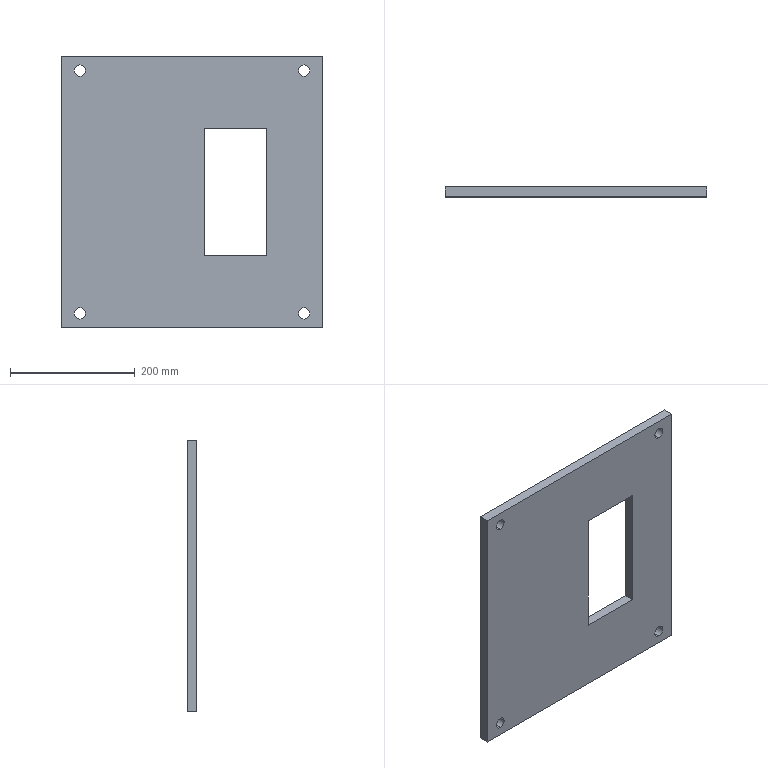Part | STEP file | 01-Base plate | 1 solid | 18 faces | box 420 x 16 x 435 mm | volume 2578914 mm3 | plane 10 | cylinder 8 | commonest cylinder face diameters 18 x8
STEP:
#1=CARTESIAN_POINT('',(0.,0.,0.));
#2=DIRECTION('',(0.,0.,1.));
#3=DIRECTION('',(1.,0.,0.));
#4=AXIS2_PLACEMENT_3D('',#1,#2,#3);
#5=CARTESIAN_POINT('',(30.,0.,421.5));
#6=VERTEX_POINT('',#5);
#7=CARTESIAN_POINT('',(30.,16.,421.5));
#8=VERTEX_POINT('',#7);
#9=CARTESIAN_POINT('',(30.,-14.,421.5));
#10=DIRECTION('',(0.,1.,0.));
#11=VECTOR('',#10,1.);
#12=LINE('',#9,#11);
#13=CARTESIAN_POINT('',(30.,-14.,412.5));
#14=DIRECTION('',(0.,1.,0.));
#15=DIRECTION('',(0.,0.,1.));
#16=AXIS2_PLACEMENT_3D('',#13,#14,#15);
#17=CYLINDRICAL_SURFACE('',#16,9.);
#18=CARTESIAN_POINT('',(6.283,0.));
#19=DIRECTION('',(0.,1.));
#20=VECTOR('',#19,1.);
#21=LINE('',#18,#20);
#22=(GEOMETRIC_REPRESENTATION_CONTEXT(2)PARAMETRIC_REPRESENTATION_CONTEXT()REPRESENTATION_CONTEXT('',''));
#23=DEFINITIONAL_REPRESENTATION('',(#21),#22);
#24=PCURVE('',#17,#23);
#25=CARTESIAN_POINT('',(30.,-14.,412.5));
#26=DIRECTION('',(0.,1.,0.));
#27=DIRECTION('',(0.,0.,1.));
#28=AXIS2_PLACEMENT_3D('',#25,#26,#27);
#29=CYLINDRICAL_SURFACE('',#28,9.);
#30=CARTESIAN_POINT('',(0.,0.));
#31=DIRECTION('',(0.,1.));
#32=VECTOR('',#31,1.);
#33=LINE('',#30,#32);
#34=(GEOMETRIC_REPRESENTATION_CONTEXT(2)PARAMETRIC_REPRESENTATION_CONTEXT()REPRESENTATION_CONTEXT('',''));
#35=DEFINITIONAL_REPRESENTATION('',(#33),#34);
#36=PCURVE('',#29,#35);
#37=SURFACE_CURVE('',#12,(#24,#36),.PCURVE_S1.);
#38=EDGE_CURVE('',#6,#8,#37,.T.);
#39=ORIENTED_EDGE('',*,*,#38,.T.);
#40=CARTESIAN_POINT('',(30.,16.,403.5));
#41=VERTEX_POINT('',#40);
#42=CARTESIAN_POINT('',(30.,16.,412.5));
#43=DIRECTION('',(0.,1.,0.));
#44=DIRECTION('',(0.,0.,1.));
#45=AXIS2_PLACEMENT_3D('',#42,#43,#44);
#46=CIRCLE('',#45,9.);
#47=CARTESIAN_POINT('',(0.,30.));
#48=DIRECTION('',(1.,0.));
#49=VECTOR('',#48,1.);
#50=LINE('',#47,#49);
#51=(GEOMETRIC_REPRESENTATION_CONTEXT(2)PARAMETRIC_REPRESENTATION_CONTEXT()REPRESENTATION_CONTEXT('',''));
#52=DEFINITIONAL_REPRESENTATION('',(#50),#51);
#53=PCURVE('',#17,#52);
#54=CARTESIAN_POINT('',(0.,16.,0.));
#55=DIRECTION('',(0.,1.,0.));
#56=DIRECTION('',(0.,0.,1.));
#57=AXIS2_PLACEMENT_3D('',#54,#55,#56);
#58=PLANE('',#57);
#59=CARTESIAN_POINT('',(412.5,30.));
#60=DIRECTION('',(1.,0.));
#61=AXIS2_PLACEMENT_2D('',#59,#60);
#62=CIRCLE('',#61,9.);
#63=(GEOMETRIC_REPRESENTATION_CONTEXT(2)PARAMETRIC_REPRESENTATION_CONTEXT()REPRESENTATION_CONTEXT('',''));
#64=DEFINITIONAL_REPRESENTATION('',(#62),#63);
#65=PCURVE('',#58,#64);
#66=SURFACE_CURVE('',#46,(#53,#65),.PCURVE_S1.);
#67=EDGE_CURVE('',#41,#8,#66,.T.);
#68=ORIENTED_EDGE('',*,*,#67,.F.);
#69=CARTESIAN_POINT('',(30.,0.,403.5));
#70=VERTEX_POINT('',#69);
#71=CARTESIAN_POINT('',(30.,-14.,403.5));
#72=DIRECTION('',(0.,1.,0.));
#73=VECTOR('',#72,1.);
#74=LINE('',#71,#73);
#75=CARTESIAN_POINT('',(3.142,0.));
#76=DIRECTION('',(0.,1.));
#77=VECTOR('',#76,1.);
#78=LINE('',#75,#77);
#79=(GEOMETRIC_REPRESENTATION_CONTEXT(2)PARAMETRIC_REPRESENTATION_CONTEXT()REPRESENTATION_CONTEXT('',''));
#80=DEFINITIONAL_REPRESENTATION('',(#78),#79);
#81=PCURVE('',#17,#80);
#82=CARTESIAN_POINT('',(3.142,0.));
#83=DIRECTION('',(0.,1.));
#84=VECTOR('',#83,1.);
#85=LINE('',#82,#84);
#86=(GEOMETRIC_REPRESENTATION_CONTEXT(2)PARAMETRIC_REPRESENTATION_CONTEXT()REPRESENTATION_CONTEXT('',''));
#87=DEFINITIONAL_REPRESENTATION('',(#85),#86);
#88=PCURVE('',#29,#87);
#89=SURFACE_CURVE('',#74,(#81,#88),.PCURVE_S1.);
#90=EDGE_CURVE('',#70,#41,#89,.T.);
#91=ORIENTED_EDGE('',*,*,#90,.F.);
#92=CARTESIAN_POINT('',(30.,0.,412.5));
#93=DIRECTION('',(0.,1.,0.));
#94=DIRECTION('',(0.,0.,1.));
#95=AXIS2_PLACEMENT_3D('',#92,#93,#94);
#96=CIRCLE('',#95,9.);
#97=CARTESIAN_POINT('',(0.,14.));
#98=DIRECTION('',(1.,0.));
#99=VECTOR('',#98,1.);
#100=LINE('',#97,#99);
#101=(GEOMETRIC_REPRESENTATION_CONTEXT(2)PARAMETRIC_REPRESENTATION_CONTEXT()REPRESENTATION_CONTEXT('',''));
#102=DEFINITIONAL_REPRESENTATION('',(#100),#101);
#103=PCURVE('',#17,#102);
#104=CARTESIAN_POINT('',(0.,0.,0.));
#105=DIRECTION('',(0.,1.,0.));
#106=DIRECTION('',(0.,0.,1.));
#107=AXIS2_PLACEMENT_3D('',#104,#105,#106);
#108=PLANE('',#107);
#109=CARTESIAN_POINT('',(412.5,30.));
#110=DIRECTION('',(1.,0.));
#111=AXIS2_PLACEMENT_2D('',#109,#110);
#112=CIRCLE('',#111,9.);
#113=(GEOMETRIC_REPRESENTATION_CONTEXT(2)PARAMETRIC_REPRESENTATION_CONTEXT()REPRESENTATION_CONTEXT('',''));
#114=DEFINITIONAL_REPRESENTATION('',(#112),#113);
#115=PCURVE('',#108,#114);
#116=SURFACE_CURVE('',#96,(#103,#115),.PCURVE_S1.);
#117=EDGE_CURVE('',#70,#6,#116,.T.);
#118=ORIENTED_EDGE('',*,*,#117,.T.);
#119=EDGE_LOOP('',(#39,#68,#91,#118));
#120=FACE_BOUND('',#119,.F.);
#121=ADVANCED_FACE('',(#120),#17,.F.);
#122=CARTESIAN_POINT('',(390.,0.,421.5));
#123=VERTEX_POINT('',#122);
#124=CARTESIAN_POINT('',(390.,16.,421.5));
#125=VERTEX_POINT('',#124);
#126=CARTESIAN_POINT('',(390.,-14.,421.5));
#127=DIRECTION('',(0.,1.,0.));
#128=VECTOR('',#127,1.);
#129=LINE('',#126,#128);
#130=CARTESIAN_POINT('',(390.,-14.,412.5));
#131=DIRECTION('',(0.,1.,0.));
#132=DIRECTION('',(0.,0.,1.));
#133=AXIS2_PLACEMENT_3D('',#130,#131,#132);
#134=CYLINDRICAL_SURFACE('',#133,9.);
#135=CARTESIAN_POINT('',(6.283,0.));
#136=DIRECTION('',(0.,1.));
#137=VECTOR('',#136,1.);
#138=LINE('',#135,#137);
#139=(GEOMETRIC_REPRESENTATION_CONTEXT(2)PARAMETRIC_REPRESENTATION_CONTEXT()REPRESENTATION_CONTEXT('',''));
#140=DEFINITIONAL_REPRESENTATION('',(#138),#139);
#141=PCURVE('',#134,#140);
#142=CARTESIAN_POINT('',(390.,-14.,412.5));
#143=DIRECTION('',(0.,1.,0.));
#144=DIRECTION('',(0.,0.,1.));
#145=AXIS2_PLACEMENT_3D('',#142,#143,#144);
#146=CYLINDRICAL_SURFACE('',#145,9.);
#147=CARTESIAN_POINT('',(0.,0.));
#148=DIRECTION('',(0.,1.));
#149=VECTOR('',#148,1.);
#150=LINE('',#147,#149);
#151=(GEOMETRIC_REPRESENTATION_CONTEXT(2)PARAMETRIC_REPRESENTATION_CONTEXT()REPRESENTATION_CONTEXT('',''));
#152=DEFINITIONAL_REPRESENTATION('',(#150),#151);
#153=PCURVE('',#146,#152);
#154=SURFACE_CURVE('',#129,(#141,#153),.PCURVE_S1.);
#155=EDGE_CURVE('',#123,#125,#154,.T.);
#156=ORIENTED_EDGE('',*,*,#155,.T.);
#157=CARTESIAN_POINT('',(390.,16.,403.5));
#158=VERTEX_POINT('',#157);
#159=CARTESIAN_POINT('',(390.,16.,412.5));
#160=DIRECTION('',(0.,1.,0.));
#161=DIRECTION('',(0.,0.,1.));
#162=AXIS2_PLACEMENT_3D('',#159,#160,#161);
#163=CIRCLE('',#162,9.);
#164=CARTESIAN_POINT('',(0.,30.));
#165=DIRECTION('',(1.,0.));
#166=VECTOR('',#165,1.);
#167=LINE('',#164,#166);
#168=(GEOMETRIC_REPRESENTATION_CONTEXT(2)PARAMETRIC_REPRESENTATION_CONTEXT()REPRESENTATION_CONTEXT('',''));
#169=DEFINITIONAL_REPRESENTATION('',(#167),#168);
#170=PCURVE('',#134,#169);
#171=CARTESIAN_POINT('',(412.5,390.));
#172=DIRECTION('',(1.,0.));
#173=AXIS2_PLACEMENT_2D('',#171,#172);
#174=CIRCLE('',#173,9.);
#175=(GEOMETRIC_REPRESENTATION_CONTEXT(2)PARAMETRIC_REPRESENTATION_CONTEXT()REPRESENTATION_CONTEXT('',''));
#176=DEFINITIONAL_REPRESENTATION('',(#174),#175);
#177=PCURVE('',#58,#176);
#178=SURFACE_CURVE('',#163,(#170,#177),.PCURVE_S1.);
#179=EDGE_CURVE('',#158,#125,#178,.T.);
#180=ORIENTED_EDGE('',*,*,#179,.F.);
#181=CARTESIAN_POINT('',(390.,0.,403.5));
#182=VERTEX_POINT('',#181);
#183=CARTESIAN_POINT('',(390.,-14.,403.5));
#184=DIRECTION('',(0.,1.,0.));
#185=VECTOR('',#184,1.);
#186=LINE('',#183,#185);
#187=CARTESIAN_POINT('',(3.142,0.));
#188=DIRECTION('',(0.,1.));
#189=VECTOR('',#188,1.);
#190=LINE('',#187,#189);
#191=(GEOMETRIC_REPRESENTATION_CONTEXT(2)PARAMETRIC_REPRESENTATION_CONTEXT()REPRESENTATION_CONTEXT('',''));
#192=DEFINITIONAL_REPRESENTATION('',(#190),#191);
#193=PCURVE('',#134,#192);
#194=CARTESIAN_POINT('',(3.142,0.));
#195=DIRECTION('',(0.,1.));
#196=VECTOR('',#195,1.);
#197=LINE('',#194,#196);
#198=(GEOMETRIC_REPRESENTATION_CONTEXT(2)PARAMETRIC_REPRESENTATION_CONTEXT()REPRESENTATION_CONTEXT('',''));
#199=DEFINITIONAL_REPRESENTATION('',(#197),#198);
#200=PCURVE('',#146,#199);
#201=SURFACE_CURVE('',#186,(#193,#200),.PCURVE_S1.);
#202=EDGE_CURVE('',#182,#158,#201,.T.);
#203=ORIENTED_EDGE('',*,*,#202,.F.);
#204=CARTESIAN_POINT('',(390.,0.,412.5));
#205=DIRECTION('',(0.,1.,0.));
#206=DIRECTION('',(0.,0.,1.));
#207=AXIS2_PLACEMENT_3D('',#204,#205,#206);
#208=CIRCLE('',#207,9.);
#209=CARTESIAN_POINT('',(0.,14.));
#210=DIRECTION('',(1.,0.));
#211=VECTOR('',#210,1.);
#212=LINE('',#209,#211);
#213=(GEOMETRIC_REPRESENTATION_CONTEXT(2)PARAMETRIC_REPRESENTATION_CONTEXT()REPRESENTATION_CONTEXT('',''));
#214=DEFINITIONAL_REPRESENTATION('',(#212),#213);
#215=PCURVE('',#134,#214);
#216=CARTESIAN_POINT('',(412.5,390.));
#217=DIRECTION('',(1.,0.));
#218=AXIS2_PLACEMENT_2D('',#216,#217);
#219=CIRCLE('',#218,9.);
#220=(GEOMETRIC_REPRESENTATION_CONTEXT(2)PARAMETRIC_REPRESENTATION_CONTEXT()REPRESENTATION_CONTEXT('',''));
#221=DEFINITIONAL_REPRESENTATION('',(#219),#220);
#222=PCURVE('',#108,#221);
#223=SURFACE_CURVE('',#208,(#215,#222),.PCURVE_S1.);
#224=EDGE_CURVE('',#182,#123,#223,.T.);
#225=ORIENTED_EDGE('',*,*,#224,.T.);
#226=EDGE_LOOP('',(#156,#180,#203,#225));
#227=FACE_BOUND('',#226,.F.);
#228=ADVANCED_FACE('',(#227),#134,.F.);
#229=CARTESIAN_POINT('',(390.,0.,31.5));
#230=VERTEX_POINT('',#229);
#231=CARTESIAN_POINT('',(390.,16.,31.5));
#232=VERTEX_POINT('',#231);
#233=CARTESIAN_POINT('',(390.,-14.,31.5));
#234=DIRECTION('',(0.,1.,0.));
#235=VECTOR('',#234,1.);
#236=LINE('',#233,#235);
#237=CARTESIAN_POINT('',(390.,-14.,22.5));
#238=DIRECTION('',(0.,1.,0.));
#239=DIRECTION('',(0.,0.,1.));
#240=AXIS2_PLACEMENT_3D('',#237,#238,#239);
#241=CYLINDRICAL_SURFACE('',#240,9.);
#242=CARTESIAN_POINT('',(6.283,0.));
#243=DIRECTION('',(0.,1.));
#244=VECTOR('',#243,1.);
#245=LINE('',#242,#244);
#246=(GEOMETRIC_REPRESENTATION_CONTEXT(2)PARAMETRIC_REPRESENTATION_CONTEXT()REPRESENTATION_CONTEXT('',''));
#247=DEFINITIONAL_REPRESENTATION('',(#245),#246);
#248=PCURVE('',#241,#247);
#249=CARTESIAN_POINT('',(390.,-14.,22.5));
#250=DIRECTION('',(0.,1.,0.));
#251=DIRECTION('',(0.,0.,1.));
#252=AXIS2_PLACEMENT_3D('',#249,#250,#251);
#253=CYLINDRICAL_SURFACE('',#252,9.);
#254=CARTESIAN_POINT('',(0.,0.));
#255=DIRECTION('',(0.,1.));
#256=VECTOR('',#255,1.);
#257=LINE('',#254,#256);
#258=(GEOMETRIC_REPRESENTATION_CONTEXT(2)PARAMETRIC_REPRESENTATION_CONTEXT()REPRESENTATION_CONTEXT('',''));
#259=DEFINITIONAL_REPRESENTATION('',(#257),#258);
#260=PCURVE('',#253,#259);
#261=SURFACE_CURVE('',#236,(#248,#260),.PCURVE_S1.);
#262=EDGE_CURVE('',#230,#232,#261,.T.);
#263=ORIENTED_EDGE('',*,*,#262,.T.);
#264=CARTESIAN_POINT('',(390.,16.,13.5));
#265=VERTEX_POINT('',#264);
#266=CARTESIAN_POINT('',(390.,16.,22.5));
#267=DIRECTION('',(0.,1.,0.));
#268=DIRECTION('',(0.,0.,1.));
#269=AXIS2_PLACEMENT_3D('',#266,#267,#268);
#270=CIRCLE('',#269,9.);
#271=CARTESIAN_POINT('',(0.,30.));
#272=DIRECTION('',(1.,0.));
#273=VECTOR('',#272,1.);
#274=LINE('',#271,#273);
#275=(GEOMETRIC_REPRESENTATION_CONTEXT(2)PARAMETRIC_REPRESENTATION_CONTEXT()REPRESENTATION_CONTEXT('',''));
#276=DEFINITIONAL_REPRESENTATION('',(#274),#275);
#277=PCURVE('',#241,#276);
#278=CARTESIAN_POINT('',(22.5,390.));
#279=DIRECTION('',(1.,0.));
#280=AXIS2_PLACEMENT_2D('',#278,#279);
#281=CIRCLE('',#280,9.);
#282=(GEOMETRIC_REPRESENTATION_CONTEXT(2)PARAMETRIC_REPRESENTATION_CONTEXT()REPRESENTATION_CONTEXT('',''));
#283=DEFINITIONAL_REPRESENTATION('',(#281),#282);
#284=PCURVE('',#58,#283);
#285=SURFACE_CURVE('',#270,(#277,#284),.PCURVE_S1.);
#286=EDGE_CURVE('',#265,#232,#285,.T.);
#287=ORIENTED_EDGE('',*,*,#286,.F.);
#288=CARTESIAN_POINT('',(390.,0.,13.5));
#289=VERTEX_POINT('',#288);
#290=CARTESIAN_POINT('',(390.,-14.,13.5));
#291=DIRECTION('',(0.,1.,0.));
#292=VECTOR('',#291,1.);
#293=LINE('',#290,#292);
#294=CARTESIAN_POINT('',(3.142,0.));
#295=DIRECTION('',(0.,1.));
#296=VECTOR('',#295,1.);
#297=LINE('',#294,#296);
#298=(GEOMETRIC_REPRESENTATION_CONTEXT(2)PARAMETRIC_REPRESENTATION_CONTEXT()REPRESENTATION_CONTEXT('',''));
#299=DEFINITIONAL_REPRESENTATION('',(#297),#298);
#300=PCURVE('',#241,#299);
#301=CARTESIAN_POINT('',(3.142,0.));
#302=DIRECTION('',(0.,1.));
#303=VECTOR('',#302,1.);
#304=LINE('',#301,#303);
#305=(GEOMETRIC_REPRESENTATION_CONTEXT(2)PARAMETRIC_REPRESENTATION_CONTEXT()REPRESENTATION_CONTEXT('',''));
#306=DEFINITIONAL_REPRESENTATION('',(#304),#305);
#307=PCURVE('',#253,#306);
#308=SURFACE_CURVE('',#293,(#300,#307),.PCURVE_S1.);
#309=EDGE_CURVE('',#289,#265,#308,.T.);
#310=ORIENTED_EDGE('',*,*,#309,.F.);
#311=CARTESIAN_POINT('',(390.,0.,22.5));
#312=DIRECTION('',(0.,1.,0.));
#313=DIRECTION('',(0.,0.,1.));
#314=AXIS2_PLACEMENT_3D('',#311,#312,#313);
#315=CIRCLE('',#314,9.);
#316=CARTESIAN_POINT('',(0.,14.));
#317=DIRECTION('',(1.,0.));
#318=VECTOR('',#317,1.);
#319=LINE('',#316,#318);
#320=(GEOMETRIC_REPRESENTATION_CONTEXT(2)PARAMETRIC_REPRESENTATION_CONTEXT()REPRESENTATION_CONTEXT('',''));
#321=DEFINITIONAL_REPRESENTATION('',(#319),#320);
#322=PCURVE('',#241,#321);
#323=CARTESIAN_POINT('',(22.5,390.));
#324=DIRECTION('',(1.,0.));
#325=AXIS2_PLACEMENT_2D('',#323,#324);
#326=CIRCLE('',#325,9.);
#327=(GEOMETRIC_REPRESENTATION_CONTEXT(2)PARAMETRIC_REPRESENTATION_CONTEXT()REPRESENTATION_CONTEXT('',''));
#328=DEFINITIONAL_REPRESENTATION('',(#326),#327);
#329=PCURVE('',#108,#328);
#330=SURFACE_CURVE('',#315,(#322,#329),.PCURVE_S1.);
#331=EDGE_CURVE('',#289,#230,#330,.T.);
#332=ORIENTED_EDGE('',*,*,#331,.T.);
#333=EDGE_LOOP('',(#263,#287,#310,#332));
#334=FACE_BOUND('',#333,.F.);
#335=ADVANCED_FACE('',(#334),#241,.F.);
#336=CARTESIAN_POINT('',(30.,0.,31.5));
#337=VERTEX_POINT('',#336);
#338=CARTESIAN_POINT('',(30.,16.,31.5));
#339=VERTEX_POINT('',#338);
#340=CARTESIAN_POINT('',(30.,-14.,31.5));
#341=DIRECTION('',(0.,1.,0.));
#342=VECTOR('',#341,1.);
#343=LINE('',#340,#342);
#344=CARTESIAN_POINT('',(30.,-14.,22.5));
#345=DIRECTION('',(0.,1.,0.));
#346=DIRECTION('',(0.,0.,1.));
#347=AXIS2_PLACEMENT_3D('',#344,#345,#346);
#348=CYLINDRICAL_SURFACE('',#347,9.);
#349=CARTESIAN_POINT('',(6.283,0.));
#350=DIRECTION('',(0.,1.));
#351=VECTOR('',#350,1.);
#352=LINE('',#349,#351);
#353=(GEOMETRIC_REPRESENTATION_CONTEXT(2)PARAMETRIC_REPRESENTATION_CONTEXT()REPRESENTATION_CONTEXT('',''));
#354=DEFINITIONAL_REPRESENTATION('',(#352),#353);
#355=PCURVE('',#348,#354);
#356=CARTESIAN_POINT('',(30.,-14.,22.5));
#357=DIRECTION('',(0.,1.,0.));
#358=DIRECTION('',(0.,0.,1.));
#359=AXIS2_PLACEMENT_3D('',#356,#357,#358);
#360=CYLINDRICAL_SURFACE('',#359,9.);
#361=CARTESIAN_POINT('',(0.,0.));
#362=DIRECTION('',(0.,1.));
#363=VECTOR('',#362,1.);
#364=LINE('',#361,#363);
#365=(GEOMETRIC_REPRESENTATION_CONTEXT(2)PARAMETRIC_REPRESENTATION_CONTEXT()REPRESENTATION_CONTEXT('',''));
#366=DEFINITIONAL_REPRESENTATION('',(#364),#365);
#367=PCURVE('',#360,#366);
#368=SURFACE_CURVE('',#343,(#355,#367),.PCURVE_S1.);
#369=EDGE_CURVE('',#337,#339,#368,.T.);
#370=ORIENTED_EDGE('',*,*,#369,.T.);
#371=CARTESIAN_POINT('',(30.,16.,13.5));
#372=VERTEX_POINT('',#371);
#373=CARTESIAN_POINT('',(30.,16.,22.5));
#374=DIRECTION('',(0.,1.,0.));
#375=DIRECTION('',(0.,0.,1.));
#376=AXIS2_PLACEMENT_3D('',#373,#374,#375);
#377=CIRCLE('',#376,9.);
#378=CARTESIAN_POINT('',(0.,30.));
#379=DIRECTION('',(1.,0.));
#380=VECTOR('',#379,1.);
#381=LINE('',#378,#380);
#382=(GEOMETRIC_REPRESENTATION_CONTEXT(2)PARAMETRIC_REPRESENTATION_CONTEXT()REPRESENTATION_CONTEXT('',''));
#383=DEFINITIONAL_REPRESENTATION('',(#381),#382);
#384=PCURVE('',#348,#383);
#385=CARTESIAN_POINT('',(22.5,30.));
#386=DIRECTION('',(1.,0.));
#387=AXIS2_PLACEMENT_2D('',#385,#386);
#388=CIRCLE('',#387,9.);
#389=(GEOMETRIC_REPRESENTATION_CONTEXT(2)PARAMETRIC_REPRESENTATION_CONTEXT()REPRESENTATION_CONTEXT('',''));
#390=DEFINITIONAL_REPRESENTATION('',(#388),#389);
#391=PCURVE('',#58,#390);
#392=SURFACE_CURVE('',#377,(#384,#391),.PCURVE_S1.);
#393=EDGE_CURVE('',#372,#339,#392,.T.);
#394=ORIENTED_EDGE('',*,*,#393,.F.);
#395=CARTESIAN_POINT('',(30.,0.,13.5));
#396=VERTEX_POINT('',#395);
#397=CARTESIAN_POINT('',(30.,-14.,13.5));
#398=DIRECTION('',(0.,1.,0.));
#399=VECTOR('',#398,1.);
#400=LINE('',#397,#399);
#401=CARTESIAN_POINT('',(3.142,0.));
#402=DIRECTION('',(0.,1.));
#403=VECTOR('',#402,1.);
#404=LINE('',#401,#403);
#405=(GEOMETRIC_REPRESENTATION_CONTEXT(2)PARAMETRIC_REPRESENTATION_CONTEXT()REPRESENTATION_CONTEXT('',''));
#406=DEFINITIONAL_REPRESENTATION('',(#404),#405);
#407=PCURVE('',#348,#406);
#408=CARTESIAN_POINT('',(3.142,0.));
#409=DIRECTION('',(0.,1.));
#410=VECTOR('',#409,1.);
#411=LINE('',#408,#410);
#412=(GEOMETRIC_REPRESENTATION_CONTEXT(2)PARAMETRIC_REPRESENTATION_CONTEXT()REPRESENTATION_CONTEXT('',''));
#413=DEFINITIONAL_REPRESENTATION('',(#411),#412);
#414=PCURVE('',#360,#413);
#415=SURFACE_CURVE('',#400,(#407,#414),.PCURVE_S1.);
#416=EDGE_CURVE('',#396,#372,#415,.T.);
#417=ORIENTED_EDGE('',*,*,#416,.F.);
#418=CARTESIAN_POINT('',(30.,0.,22.5));
#419=DIRECTION('',(0.,1.,0.));
#420=DIRECTION('',(0.,0.,1.));
#421=AXIS2_PLACEMENT_3D('',#418,#419,#420);
#422=CIRCLE('',#421,9.);
#423=CARTESIAN_POINT('',(0.,14.));
#424=DIRECTION('',(1.,0.));
#425=VECTOR('',#424,1.);
#426=LINE('',#423,#425);
#427=(GEOMETRIC_REPRESENTATION_CONTEXT(2)PARAMETRIC_REPRESENTATION_CONTEXT()REPRESENTATION_CONTEXT('',''));
#428=DEFINITIONAL_REPRESENTATION('',(#426),#427);
#429=PCURVE('',#348,#428);
#430=CARTESIAN_POINT('',(22.5,30.));
#431=DIRECTION('',(1.,0.));
#432=AXIS2_PLACEMENT_2D('',#430,#431);
#433=CIRCLE('',#432,9.);
#434=(GEOMETRIC_REPRESENTATION_CONTEXT(2)PARAMETRIC_REPRESENTATION_CONTEXT()REPRESENTATION_CONTEXT('',''));
#435=DEFINITIONAL_REPRESENTATION('',(#433),#434);
#436=PCURVE('',#108,#435);
#437=SURFACE_CURVE('',#422,(#429,#436),.PCURVE_S1.);
#438=EDGE_CURVE('',#396,#337,#437,.T.);
#439=ORIENTED_EDGE('',*,*,#438,.T.);
#440=EDGE_LOOP('',(#370,#394,#417,#439));
#441=FACE_BOUND('',#440,.F.);
#442=ADVANCED_FACE('',(#441),#348,.F.);
#443=CARTESIAN_POINT('',(0.,0.,0.));
#444=VERTEX_POINT('',#443);
#445=CARTESIAN_POINT('',(0.,0.,435.));
#446=VERTEX_POINT('',#445);
#447=CARTESIAN_POINT('',(0.,0.,0.));
#448=DIRECTION('',(0.,0.,1.));
#449=VECTOR('',#448,1.);
#450=LINE('',#447,#449);
#451=CARTESIAN_POINT('',(0.,16.,0.));
#452=DIRECTION('',(1.,0.,0.));
#453=DIRECTION('',(0.,0.,-1.));
#454=AXIS2_PLACEMENT_3D('',#451,#452,#453);
#455=PLANE('',#454);
#456=CARTESIAN_POINT('',(0.,-16.));
#457=DIRECTION('',(-1.,0.));
#458=VECTOR('',#457,1.);
#459=LINE('',#456,#458);
#460=(GEOMETRIC_REPRESENTATION_CONTEXT(2)PARAMETRIC_REPRESENTATION_CONTEXT()REPRESENTATION_CONTEXT('',''));
#461=DEFINITIONAL_REPRESENTATION('',(#459),#460);
#462=PCURVE('',#455,#461);
#463=CARTESIAN_POINT('',(0.,0.));
#464=DIRECTION('',(1.,0.));
#465=VECTOR('',#464,1.);
#466=LINE('',#463,#465);
#467=(GEOMETRIC_REPRESENTATION_CONTEXT(2)PARAMETRIC_REPRESENTATION_CONTEXT()REPRESENTATION_CONTEXT('',''));
#468=DEFINITIONAL_REPRESENTATION('',(#466),#467);
#469=PCURVE('',#108,#468);
#470=SURFACE_CURVE('',#450,(#462,#469),.PCURVE_S1.);
#471=EDGE_CURVE('',#444,#446,#470,.T.);
#472=ORIENTED_EDGE('',*,*,#471,.T.);
#473=CARTESIAN_POINT('',(0.,16.,435.));
#474=VERTEX_POINT('',#473);
#475=CARTESIAN_POINT('',(0.,16.,435.));
#476=DIRECTION('',(0.,-1.,0.));
#477=VECTOR('',#476,1.);
#478=LINE('',#475,#477);
#479=CARTESIAN_POINT('',(-435.,0.));
#480=DIRECTION('',(0.,-1.));
#481=VECTOR('',#480,1.);
#482=LINE('',#479,#481);
#483=(GEOMETRIC_REPRESENTATION_CONTEXT(2)PARAMETRIC_REPRESENTATION_CONTEXT()REPRESENTATION_CONTEXT('',''));
#484=DEFINITIONAL_REPRESENTATION('',(#482),#483);
#485=PCURVE('',#455,#484);
#486=CARTESIAN_POINT('',(0.,16.,435.));
#487=DIRECTION('',(0.,0.,-1.));
#488=DIRECTION('',(-1.,0.,0.));
#489=AXIS2_PLACEMENT_3D('',#486,#487,#488);
#490=PLANE('',#489);
#491=CARTESIAN_POINT('',(0.,0.));
#492=DIRECTION('',(0.,-1.));
#493=VECTOR('',#492,1.);
#494=LINE('',#491,#493);
#495=(GEOMETRIC_REPRESENTATION_CONTEXT(2)PARAMETRIC_REPRESENTATION_CONTEXT()REPRESENTATION_CONTEXT('',''));
#496=DEFINITIONAL_REPRESENTATION('',(#494),#495);
#497=PCURVE('',#490,#496);
#498=SURFACE_CURVE('',#478,(#485,#497),.PCURVE_S1.);
#499=EDGE_CURVE('',#474,#446,#498,.T.);
#500=ORIENTED_EDGE('',*,*,#499,.F.);
#501=CARTESIAN_POINT('',(0.,16.,0.));
#502=VERTEX_POINT('',#501);
#503=CARTESIAN_POINT('',(0.,16.,0.));
#504=DIRECTION('',(0.,0.,1.));
#505=VECTOR('',#504,1.);
#506=LINE('',#503,#505);
#507=CARTESIAN_POINT('',(0.,0.));
#508=DIRECTION('',(-1.,0.));
#509=VECTOR('',#508,1.);
#510=LINE('',#507,#509);
#511=(GEOMETRIC_REPRESENTATION_CONTEXT(2)PARAMETRIC_REPRESENTATION_CONTEXT()REPRESENTATION_CONTEXT('',''));
#512=DEFINITIONAL_REPRESENTATION('',(#510),#511);
#513=PCURVE('',#455,#512);
#514=CARTESIAN_POINT('',(0.,0.));
#515=DIRECTION('',(1.,0.));
#516=VECTOR('',#515,1.);
#517=LINE('',#514,#516);
#518=(GEOMETRIC_REPRESENTATION_CONTEXT(2)PARAMETRIC_REPRESENTATION_CONTEXT()REPRESENTATION_CONTEXT('',''));
#519=DEFINITIONAL_REPRESENTATION('',(#517),#518);
#520=PCURVE('',#58,#519);
#521=SURFACE_CURVE('',#506,(#513,#520),.PCURVE_S1.);
#522=EDGE_CURVE('',#502,#474,#521,.T.);
#523=ORIENTED_EDGE('',*,*,#522,.F.);
#524=CARTESIAN_POINT('',(0.,16.,0.));
#525=DIRECTION('',(0.,-1.,0.));
#526=VECTOR('',#525,1.);
#527=LINE('',#524,#526);
#528=CARTESIAN_POINT('',(0.,0.));
#529=DIRECTION('',(0.,-1.));
#530=VECTOR('',#529,1.);
#531=LINE('',#528,#530);
#532=(GEOMETRIC_REPRESENTATION_CONTEXT(2)PARAMETRIC_REPRESENTATION_CONTEXT()REPRESENTATION_CONTEXT('',''));
#533=DEFINITIONAL_REPRESENTATION('',(#531),#532);
#534=PCURVE('',#455,#533);
#535=CARTESIAN_POINT('',(0.,16.,0.));
#536=DIRECTION('',(0.,0.,1.));
#537=DIRECTION('',(1.,0.,0.));
#538=AXIS2_PLACEMENT_3D('',#535,#536,#537);
#539=PLANE('',#538);
#540=CARTESIAN_POINT('',(0.,0.));
#541=DIRECTION('',(0.,-1.));
#542=VECTOR('',#541,1.);
#543=LINE('',#540,#542);
#544=(GEOMETRIC_REPRESENTATION_CONTEXT(2)PARAMETRIC_REPRESENTATION_CONTEXT()REPRESENTATION_CONTEXT('',''));
#545=DEFINITIONAL_REPRESENTATION('',(#543),#544);
#546=PCURVE('',#539,#545);
#547=SURFACE_CURVE('',#527,(#534,#546),.PCURVE_S1.);
#548=EDGE_CURVE('',#502,#444,#547,.T.);
#549=ORIENTED_EDGE('',*,*,#548,.T.);
#550=EDGE_LOOP('',(#472,#500,#523,#549));
#551=FACE_BOUND('',#550,.T.);
#552=ADVANCED_FACE('',(#551),#455,.F.);
#553=CARTESIAN_POINT('',(420.,0.,435.));
#554=VERTEX_POINT('',#553);
#555=CARTESIAN_POINT('',(0.,0.,435.));
#556=DIRECTION('',(1.,0.,0.));
#557=VECTOR('',#556,1.);
#558=LINE('',#555,#557);
#559=CARTESIAN_POINT('',(0.,-16.));
#560=DIRECTION('',(-1.,0.));
#561=VECTOR('',#560,1.);
#562=LINE('',#559,#561);
#563=(GEOMETRIC_REPRESENTATION_CONTEXT(2)PARAMETRIC_REPRESENTATION_CONTEXT()REPRESENTATION_CONTEXT('',''));
#564=DEFINITIONAL_REPRESENTATION('',(#562),#563);
#565=PCURVE('',#490,#564);
#566=CARTESIAN_POINT('',(435.,0.));
#567=DIRECTION('',(0.,1.));
#568=VECTOR('',#567,1.);
#569=LINE('',#566,#568);
#570=(GEOMETRIC_REPRESENTATION_CONTEXT(2)PARAMETRIC_REPRESENTATION_CONTEXT()REPRESENTATION_CONTEXT('',''));
#571=DEFINITIONAL_REPRESENTATION('',(#569),#570);
#572=PCURVE('',#108,#571);
#573=SURFACE_CURVE('',#558,(#565,#572),.PCURVE_S1.);
#574=EDGE_CURVE('',#446,#554,#573,.T.);
#575=ORIENTED_EDGE('',*,*,#574,.T.);
#576=CARTESIAN_POINT('',(420.,16.,435.));
#577=VERTEX_POINT('',#576);
#578=CARTESIAN_POINT('',(420.,16.,435.));
#579=DIRECTION('',(0.,-1.,0.));
#580=VECTOR('',#579,1.);
#581=LINE('',#578,#580);
#582=CARTESIAN_POINT('',(-420.,0.));
#583=DIRECTION('',(0.,-1.));
#584=VECTOR('',#583,1.);
#585=LINE('',#582,#584);
#586=(GEOMETRIC_REPRESENTATION_CONTEXT(2)PARAMETRIC_REPRESENTATION_CONTEXT()REPRESENTATION_CONTEXT('',''));
#587=DEFINITIONAL_REPRESENTATION('',(#585),#586);
#588=PCURVE('',#490,#587);
#589=CARTESIAN_POINT('',(420.,16.,0.));
#590=DIRECTION('',(-1.,0.,0.));
#591=DIRECTION('',(0.,0.,1.));
#592=AXIS2_PLACEMENT_3D('',#589,#590,#591);
#593=PLANE('',#592);
#594=CARTESIAN_POINT('',(435.,0.));
#595=DIRECTION('',(0.,-1.));
#596=VECTOR('',#595,1.);
#597=LINE('',#594,#596);
#598=(GEOMETRIC_REPRESENTATION_CONTEXT(2)PARAMETRIC_REPRESENTATION_CONTEXT()REPRESENTATION_CONTEXT('',''));
#599=DEFINITIONAL_REPRESENTATION('',(#597),#598);
#600=PCURVE('',#593,#599);
#601=SURFACE_CURVE('',#581,(#588,#600),.PCURVE_S1.);
#602=EDGE_CURVE('',#577,#554,#601,.T.);
#603=ORIENTED_EDGE('',*,*,#602,.F.);
#604=CARTESIAN_POINT('',(0.,16.,435.));
#605=DIRECTION('',(1.,0.,0.));
#606=VECTOR('',#605,1.);
#607=LINE('',#604,#606);
#608=CARTESIAN_POINT('',(0.,0.));
#609=DIRECTION('',(-1.,0.));
#610=VECTOR('',#609,1.);
#611=LINE('',#608,#610);
#612=(GEOMETRIC_REPRESENTATION_CONTEXT(2)PARAMETRIC_REPRESENTATION_CONTEXT()REPRESENTATION_CONTEXT('',''));
#613=DEFINITIONAL_REPRESENTATION('',(#611),#612);
#614=PCURVE('',#490,#613);
#615=CARTESIAN_POINT('',(435.,0.));
#616=DIRECTION('',(0.,1.));
#617=VECTOR('',#616,1.);
#618=LINE('',#615,#617);
#619=(GEOMETRIC_REPRESENTATION_CONTEXT(2)PARAMETRIC_REPRESENTATION_CONTEXT()REPRESENTATION_CONTEXT('',''));
#620=DEFINITIONAL_REPRESENTATION('',(#618),#619);
#621=PCURVE('',#58,#620);
#622=SURFACE_CURVE('',#607,(#614,#621),.PCURVE_S1.);
#623=EDGE_CURVE('',#474,#577,#622,.T.);
#624=ORIENTED_EDGE('',*,*,#623,.F.);
#625=ORIENTED_EDGE('',*,*,#499,.T.);
#626=EDGE_LOOP('',(#575,#603,#624,#625));
#627=FACE_BOUND('',#626,.T.);
#628=ADVANCED_FACE('',(#627),#490,.F.);
#629=CARTESIAN_POINT('',(420.,0.,0.));
#630=VERTEX_POINT('',#629);
#631=CARTESIAN_POINT('',(420.,0.,0.));
#632=DIRECTION('',(0.,0.,-1.));
#633=VECTOR('',#632,1.);
#634=LINE('',#631,#633);
#635=CARTESIAN_POINT('',(0.,-16.));
#636=DIRECTION('',(-1.,0.));
#637=VECTOR('',#636,1.);
#638=LINE('',#635,#637);
#639=(GEOMETRIC_REPRESENTATION_CONTEXT(2)PARAMETRIC_REPRESENTATION_CONTEXT()REPRESENTATION_CONTEXT('',''));
#640=DEFINITIONAL_REPRESENTATION('',(#638),#639);
#641=PCURVE('',#593,#640);
#642=CARTESIAN_POINT('',(0.,420.));
#643=DIRECTION('',(-1.,0.));
#644=VECTOR('',#643,1.);
#645=LINE('',#642,#644);
#646=(GEOMETRIC_REPRESENTATION_CONTEXT(2)PARAMETRIC_REPRESENTATION_CONTEXT()REPRESENTATION_CONTEXT('',''));
#647=DEFINITIONAL_REPRESENTATION('',(#645),#646);
#648=PCURVE('',#108,#647);
#649=SURFACE_CURVE('',#634,(#641,#648),.PCURVE_S1.);
#650=EDGE_CURVE('',#554,#630,#649,.T.);
#651=ORIENTED_EDGE('',*,*,#650,.T.);
#652=CARTESIAN_POINT('',(420.,16.,0.));
#653=VERTEX_POINT('',#652);
#654=CARTESIAN_POINT('',(420.,16.,0.));
#655=DIRECTION('',(0.,-1.,0.));
#656=VECTOR('',#655,1.);
#657=LINE('',#654,#656);
#658=CARTESIAN_POINT('',(0.,0.));
#659=DIRECTION('',(0.,-1.));
#660=VECTOR('',#659,1.);
#661=LINE('',#658,#660);
#662=(GEOMETRIC_REPRESENTATION_CONTEXT(2)PARAMETRIC_REPRESENTATION_CONTEXT()REPRESENTATION_CONTEXT('',''));
#663=DEFINITIONAL_REPRESENTATION('',(#661),#662);
#664=PCURVE('',#593,#663);
#665=CARTESIAN_POINT('',(420.,0.));
#666=DIRECTION('',(0.,-1.));
#667=VECTOR('',#666,1.);
#668=LINE('',#665,#667);
#669=(GEOMETRIC_REPRESENTATION_CONTEXT(2)PARAMETRIC_REPRESENTATION_CONTEXT()REPRESENTATION_CONTEXT('',''));
#670=DEFINITIONAL_REPRESENTATION('',(#668),#669);
#671=PCURVE('',#539,#670);
#672=SURFACE_CURVE('',#657,(#664,#671),.PCURVE_S1.);
#673=EDGE_CURVE('',#653,#630,#672,.T.);
#674=ORIENTED_EDGE('',*,*,#673,.F.);
#675=CARTESIAN_POINT('',(420.,16.,0.));
#676=DIRECTION('',(0.,0.,-1.));
#677=VECTOR('',#676,1.);
#678=LINE('',#675,#677);
#679=CARTESIAN_POINT('',(0.,0.));
#680=DIRECTION('',(-1.,0.));
#681=VECTOR('',#680,1.);
#682=LINE('',#679,#681);
#683=(GEOMETRIC_REPRESENTATION_CONTEXT(2)PARAMETRIC_REPRESENTATION_CONTEXT()REPRESENTATION_CONTEXT('',''));
#684=DEFINITIONAL_REPRESENTATION('',(#682),#683);
#685=PCURVE('',#593,#684);
#686=CARTESIAN_POINT('',(0.,420.));
#687=DIRECTION('',(-1.,0.));
#688=VECTOR('',#687,1.);
#689=LINE('',#686,#688);
#690=(GEOMETRIC_REPRESENTATION_CONTEXT(2)PARAMETRIC_REPRESENTATION_CONTEXT()REPRESENTATION_CONTEXT('',''));
#691=DEFINITIONAL_REPRESENTATION('',(#689),#690);
#692=PCURVE('',#58,#691);
#693=SURFACE_CURVE('',#678,(#685,#692),.PCURVE_S1.);
#694=EDGE_CURVE('',#577,#653,#693,.T.);
#695=ORIENTED_EDGE('',*,*,#694,.F.);
#696=ORIENTED_EDGE('',*,*,#602,.T.);
#697=EDGE_LOOP('',(#651,#674,#695,#696));
#698=FACE_BOUND('',#697,.T.);
#699=ADVANCED_FACE('',(#698),#593,.F.);
#700=CARTESIAN_POINT('',(0.,0.,0.));
#701=DIRECTION('',(-1.,0.,0.));
#702=VECTOR('',#701,1.);
#703=LINE('',#700,#702);
#704=CARTESIAN_POINT('',(0.,-16.));
#705=DIRECTION('',(-1.,0.));
#706=VECTOR('',#705,1.);
#707=LINE('',#704,#706);
#708=(GEOMETRIC_REPRESENTATION_CONTEXT(2)PARAMETRIC_REPRESENTATION_CONTEXT()REPRESENTATION_CONTEXT('',''));
#709=DEFINITIONAL_REPRESENTATION('',(#707),#708);
#710=PCURVE('',#539,#709);
#711=CARTESIAN_POINT('',(0.,0.));
#712=DIRECTION('',(0.,-1.));
#713=VECTOR('',#712,1.);
#714=LINE('',#711,#713);
#715=(GEOMETRIC_REPRESENTATION_CONTEXT(2)PARAMETRIC_REPRESENTATION_CONTEXT()REPRESENTATION_CONTEXT('',''));
#716=DEFINITIONAL_REPRESENTATION('',(#714),#715);
#717=PCURVE('',#108,#716);
#718=SURFACE_CURVE('',#703,(#710,#717),.PCURVE_S1.);
#719=EDGE_CURVE('',#630,#444,#718,.T.);
#720=ORIENTED_EDGE('',*,*,#719,.T.);
#721=ORIENTED_EDGE('',*,*,#548,.F.);
#722=CARTESIAN_POINT('',(0.,16.,0.));
#723=DIRECTION('',(-1.,0.,0.));
#724=VECTOR('',#723,1.);
#725=LINE('',#722,#724);
#726=CARTESIAN_POINT('',(0.,0.));
#727=DIRECTION('',(-1.,0.));
#728=VECTOR('',#727,1.);
#729=LINE('',#726,#728);
#730=(GEOMETRIC_REPRESENTATION_CONTEXT(2)PARAMETRIC_REPRESENTATION_CONTEXT()REPRESENTATION_CONTEXT('',''));
#731=DEFINITIONAL_REPRESENTATION('',(#729),#730);
#732=PCURVE('',#539,#731);
#733=CARTESIAN_POINT('',(0.,0.));
#734=DIRECTION('',(0.,-1.));
#735=VECTOR('',#734,1.);
#736=LINE('',#733,#735);
#737=(GEOMETRIC_REPRESENTATION_CONTEXT(2)PARAMETRIC_REPRESENTATION_CONTEXT()REPRESENTATION_CONTEXT('',''));
#738=DEFINITIONAL_REPRESENTATION('',(#736),#737);
#739=PCURVE('',#58,#738);
#740=SURFACE_CURVE('',#725,(#732,#739),.PCURVE_S1.);
#741=EDGE_CURVE('',#653,#502,#740,.T.);
#742=ORIENTED_EDGE('',*,*,#741,.F.);
#743=ORIENTED_EDGE('',*,*,#673,.T.);
#744=EDGE_LOOP('',(#720,#721,#742,#743));
#745=FACE_BOUND('',#744,.T.);
#746=ADVANCED_FACE('',(#745),#539,.F.);
#747=CARTESIAN_POINT('',(230.,16.,115.));
#748=VERTEX_POINT('',#747);
#749=CARTESIAN_POINT('',(230.,16.,320.));
#750=VERTEX_POINT('',#749);
#751=CARTESIAN_POINT('',(230.,16.,115.));
#752=DIRECTION('',(0.,0.,1.));
#753=VECTOR('',#752,1.);
#754=LINE('',#751,#753);
#755=CARTESIAN_POINT('',(115.,230.));
#756=DIRECTION('',(1.,0.));
#757=VECTOR('',#756,1.);
#758=LINE('',#755,#757);
#759=(GEOMETRIC_REPRESENTATION_CONTEXT(2)PARAMETRIC_REPRESENTATION_CONTEXT()REPRESENTATION_CONTEXT('',''));
#760=DEFINITIONAL_REPRESENTATION('',(#758),#759);
#761=PCURVE('',#58,#760);
#762=CARTESIAN_POINT('',(230.,-4.,115.));
#763=DIRECTION('',(-1.,0.,0.));
#764=DIRECTION('',(0.,0.,1.));
#765=AXIS2_PLACEMENT_3D('',#762,#763,#764);
#766=PLANE('',#765);
#767=CARTESIAN_POINT('',(0.,20.));
#768=DIRECTION('',(1.,0.));
#769=VECTOR('',#768,1.);
#770=LINE('',#767,#769);
#771=(GEOMETRIC_REPRESENTATION_CONTEXT(2)PARAMETRIC_REPRESENTATION_CONTEXT()REPRESENTATION_CONTEXT('',''));
#772=DEFINITIONAL_REPRESENTATION('',(#770),#771);
#773=PCURVE('',#766,#772);
#774=SURFACE_CURVE('',#754,(#761,#773),.PCURVE_S1.);
#775=EDGE_CURVE('',#748,#750,#774,.T.);
#776=ORIENTED_EDGE('',*,*,#775,.F.);
#777=CARTESIAN_POINT('',(330.,16.,115.));
#778=VERTEX_POINT('',#777);
#779=CARTESIAN_POINT('',(230.,16.,115.));
#780=DIRECTION('',(-1.,0.,0.));
#781=VECTOR('',#780,1.);
#782=LINE('',#779,#781);
#783=CARTESIAN_POINT('',(115.,230.));
#784=DIRECTION('',(0.,-1.));
#785=VECTOR('',#784,1.);
#786=LINE('',#783,#785);
#787=(GEOMETRIC_REPRESENTATION_CONTEXT(2)PARAMETRIC_REPRESENTATION_CONTEXT()REPRESENTATION_CONTEXT('',''));
#788=DEFINITIONAL_REPRESENTATION('',(#786),#787);
#789=PCURVE('',#58,#788);
#790=CARTESIAN_POINT('',(230.,-4.,115.));
#791=DIRECTION('',(0.,0.,-1.));
#792=DIRECTION('',(-1.,0.,0.));
#793=AXIS2_PLACEMENT_3D('',#790,#791,#792);
#794=PLANE('',#793);
#795=CARTESIAN_POINT('',(0.,20.));
#796=DIRECTION('',(1.,0.));
#797=VECTOR('',#796,1.);
#798=LINE('',#795,#797);
#799=(GEOMETRIC_REPRESENTATION_CONTEXT(2)PARAMETRIC_REPRESENTATION_CONTEXT()REPRESENTATION_CONTEXT('',''));
#800=DEFINITIONAL_REPRESENTATION('',(#798),#799);
#801=PCURVE('',#794,#800);
#802=SURFACE_CURVE('',#782,(#789,#801),.PCURVE_S1.);
#803=EDGE_CURVE('',#778,#748,#802,.T.);
#804=ORIENTED_EDGE('',*,*,#803,.F.);
#805=CARTESIAN_POINT('',(330.,16.,320.));
#806=VERTEX_POINT('',#805);
#807=CARTESIAN_POINT('',(330.,16.,115.));
#808=DIRECTION('',(0.,0.,-1.));
#809=VECTOR('',#808,1.);
#810=LINE('',#807,#809);
#811=CARTESIAN_POINT('',(115.,330.));
#812=DIRECTION('',(-1.,0.));
#813=VECTOR('',#812,1.);
#814=LINE('',#811,#813);
#815=(GEOMETRIC_REPRESENTATION_CONTEXT(2)PARAMETRIC_REPRESENTATION_CONTEXT()REPRESENTATION_CONTEXT('',''));
#816=DEFINITIONAL_REPRESENTATION('',(#814),#815);
#817=PCURVE('',#58,#816);
#818=CARTESIAN_POINT('',(330.,-4.,115.));
#819=DIRECTION('',(1.,0.,0.));
#820=DIRECTION('',(0.,0.,-1.));
#821=AXIS2_PLACEMENT_3D('',#818,#819,#820);
#822=PLANE('',#821);
#823=CARTESIAN_POINT('',(0.,20.));
#824=DIRECTION('',(1.,0.));
#825=VECTOR('',#824,1.);
#826=LINE('',#823,#825);
#827=(GEOMETRIC_REPRESENTATION_CONTEXT(2)PARAMETRIC_REPRESENTATION_CONTEXT()REPRESENTATION_CONTEXT('',''));
#828=DEFINITIONAL_REPRESENTATION('',(#826),#827);
#829=PCURVE('',#822,#828);
#830=SURFACE_CURVE('',#810,(#817,#829),.PCURVE_S1.);
#831=EDGE_CURVE('',#806,#778,#830,.T.);
#832=ORIENTED_EDGE('',*,*,#831,.F.);
#833=CARTESIAN_POINT('',(230.,16.,320.));
#834=DIRECTION('',(1.,0.,0.));
#835=VECTOR('',#834,1.);
#836=LINE('',#833,#835);
#837=CARTESIAN_POINT('',(320.,230.));
#838=DIRECTION('',(0.,1.));
#839=VECTOR('',#838,1.);
#840=LINE('',#837,#839);
#841=(GEOMETRIC_REPRESENTATION_CONTEXT(2)PARAMETRIC_REPRESENTATION_CONTEXT()REPRESENTATION_CONTEXT('',''));
#842=DEFINITIONAL_REPRESENTATION('',(#840),#841);
#843=PCURVE('',#58,#842);
#844=CARTESIAN_POINT('',(230.,-4.,320.));
#845=DIRECTION('',(0.,0.,1.));
#846=DIRECTION('',(1.,0.,0.));
#847=AXIS2_PLACEMENT_3D('',#844,#845,#846);
#848=PLANE('',#847);
#849=CARTESIAN_POINT('',(0.,20.));
#850=DIRECTION('',(1.,0.));
#851=VECTOR('',#850,1.);
#852=LINE('',#849,#851);
#853=(GEOMETRIC_REPRESENTATION_CONTEXT(2)PARAMETRIC_REPRESENTATION_CONTEXT()REPRESENTATION_CONTEXT('',''));
#854=DEFINITIONAL_REPRESENTATION('',(#852),#853);
#855=PCURVE('',#848,#854);
#856=SURFACE_CURVE('',#836,(#843,#855),.PCURVE_S1.);
#857=EDGE_CURVE('',#750,#806,#856,.T.);
#858=ORIENTED_EDGE('',*,*,#857,.F.);
#859=EDGE_LOOP('',(#776,#804,#832,#858));
#860=FACE_BOUND('',#859,.T.);
#861=CARTESIAN_POINT('',(30.,16.,412.5));
#862=DIRECTION('',(0.,1.,0.));
#863=DIRECTION('',(0.,0.,1.));
#864=AXIS2_PLACEMENT_3D('',#861,#862,#863);
#865=CIRCLE('',#864,9.);
#866=CARTESIAN_POINT('',(412.5,30.));
#867=DIRECTION('',(1.,0.));
#868=AXIS2_PLACEMENT_2D('',#866,#867);
#869=CIRCLE('',#868,9.);
#870=(GEOMETRIC_REPRESENTATION_CONTEXT(2)PARAMETRIC_REPRESENTATION_CONTEXT()REPRESENTATION_CONTEXT('',''));
#871=DEFINITIONAL_REPRESENTATION('',(#869),#870);
#872=PCURVE('',#58,#871);
#873=CARTESIAN_POINT('',(0.,30.));
#874=DIRECTION('',(1.,0.));
#875=VECTOR('',#874,1.);
#876=LINE('',#873,#875);
#877=(GEOMETRIC_REPRESENTATION_CONTEXT(2)PARAMETRIC_REPRESENTATION_CONTEXT()REPRESENTATION_CONTEXT('',''));
#878=DEFINITIONAL_REPRESENTATION('',(#876),#877);
#879=PCURVE('',#29,#878);
#880=SURFACE_CURVE('',#865,(#872,#879),.PCURVE_S1.);
#881=EDGE_CURVE('',#8,#41,#880,.T.);
#882=ORIENTED_EDGE('',*,*,#881,.F.);
#883=ORIENTED_EDGE('',*,*,#67,.F.);
#884=EDGE_LOOP('',(#882,#883));
#885=FACE_BOUND('',#884,.T.);
#886=CARTESIAN_POINT('',(390.,16.,412.5));
#887=DIRECTION('',(0.,1.,0.));
#888=DIRECTION('',(0.,0.,1.));
#889=AXIS2_PLACEMENT_3D('',#886,#887,#888);
#890=CIRCLE('',#889,9.);
#891=CARTESIAN_POINT('',(412.5,390.));
#892=DIRECTION('',(1.,0.));
#893=AXIS2_PLACEMENT_2D('',#891,#892);
#894=CIRCLE('',#893,9.);
#895=(GEOMETRIC_REPRESENTATION_CONTEXT(2)PARAMETRIC_REPRESENTATION_CONTEXT()REPRESENTATION_CONTEXT('',''));
#896=DEFINITIONAL_REPRESENTATION('',(#894),#895);
#897=PCURVE('',#58,#896);
#898=CARTESIAN_POINT('',(0.,30.));
#899=DIRECTION('',(1.,0.));
#900=VECTOR('',#899,1.);
#901=LINE('',#898,#900);
#902=(GEOMETRIC_REPRESENTATION_CONTEXT(2)PARAMETRIC_REPRESENTATION_CONTEXT()REPRESENTATION_CONTEXT('',''));
#903=DEFINITIONAL_REPRESENTATION('',(#901),#902);
#904=PCURVE('',#146,#903);
#905=SURFACE_CURVE('',#890,(#897,#904),.PCURVE_S1.);
#906=EDGE_CURVE('',#125,#158,#905,.T.);
#907=ORIENTED_EDGE('',*,*,#906,.F.);
#908=ORIENTED_EDGE('',*,*,#179,.F.);
#909=EDGE_LOOP('',(#907,#908));
#910=FACE_BOUND('',#909,.T.);
#911=CARTESIAN_POINT('',(390.,16.,22.5));
#912=DIRECTION('',(0.,1.,0.));
#913=DIRECTION('',(0.,0.,1.));
#914=AXIS2_PLACEMENT_3D('',#911,#912,#913);
#915=CIRCLE('',#914,9.);
#916=CARTESIAN_POINT('',(22.5,390.));
#917=DIRECTION('',(1.,0.));
#918=AXIS2_PLACEMENT_2D('',#916,#917);
#919=CIRCLE('',#918,9.);
#920=(GEOMETRIC_REPRESENTATION_CONTEXT(2)PARAMETRIC_REPRESENTATION_CONTEXT()REPRESENTATION_CONTEXT('',''));
#921=DEFINITIONAL_REPRESENTATION('',(#919),#920);
#922=PCURVE('',#58,#921);
#923=CARTESIAN_POINT('',(0.,30.));
#924=DIRECTION('',(1.,0.));
#925=VECTOR('',#924,1.);
#926=LINE('',#923,#925);
#927=(GEOMETRIC_REPRESENTATION_CONTEXT(2)PARAMETRIC_REPRESENTATION_CONTEXT()REPRESENTATION_CONTEXT('',''));
#928=DEFINITIONAL_REPRESENTATION('',(#926),#927);
#929=PCURVE('',#253,#928);
#930=SURFACE_CURVE('',#915,(#922,#929),.PCURVE_S1.);
#931=EDGE_CURVE('',#232,#265,#930,.T.);
#932=ORIENTED_EDGE('',*,*,#931,.F.);
#933=ORIENTED_EDGE('',*,*,#286,.F.);
#934=EDGE_LOOP('',(#932,#933));
#935=FACE_BOUND('',#934,.T.);
#936=CARTESIAN_POINT('',(30.,16.,22.5));
#937=DIRECTION('',(0.,1.,0.));
#938=DIRECTION('',(0.,0.,1.));
#939=AXIS2_PLACEMENT_3D('',#936,#937,#938);
#940=CIRCLE('',#939,9.);
#941=CARTESIAN_POINT('',(22.5,30.));
#942=DIRECTION('',(1.,0.));
#943=AXIS2_PLACEMENT_2D('',#941,#942);
#944=CIRCLE('',#943,9.);
#945=(GEOMETRIC_REPRESENTATION_CONTEXT(2)PARAMETRIC_REPRESENTATION_CONTEXT()REPRESENTATION_CONTEXT('',''));
#946=DEFINITIONAL_REPRESENTATION('',(#944),#945);
#947=PCURVE('',#58,#946);
#948=CARTESIAN_POINT('',(0.,30.));
#949=DIRECTION('',(1.,0.));
#950=VECTOR('',#949,1.);
#951=LINE('',#948,#950);
#952=(GEOMETRIC_REPRESENTATION_CONTEXT(2)PARAMETRIC_REPRESENTATION_CONTEXT()REPRESENTATION_CONTEXT('',''));
#953=DEFINITIONAL_REPRESENTATION('',(#951),#952);
#954=PCURVE('',#360,#953);
#955=SURFACE_CURVE('',#940,(#947,#954),.PCURVE_S1.);
#956=EDGE_CURVE('',#339,#372,#955,.T.);
#957=ORIENTED_EDGE('',*,*,#956,.F.);
#958=ORIENTED_EDGE('',*,*,#393,.F.);
#959=EDGE_LOOP('',(#957,#958));
#960=FACE_BOUND('',#959,.T.);
#961=ORIENTED_EDGE('',*,*,#522,.T.);
#962=ORIENTED_EDGE('',*,*,#623,.T.);
#963=ORIENTED_EDGE('',*,*,#694,.T.);
#964=ORIENTED_EDGE('',*,*,#741,.T.);
#965=EDGE_LOOP('',(#961,#962,#963,#964));
#966=FACE_BOUND('',#965,.T.);
#967=ADVANCED_FACE('',(#860,#885,#910,#935,#960,#966),#58,.T.);
#968=CARTESIAN_POINT('',(330.,0.,115.));
#969=VERTEX_POINT('',#968);
#970=CARTESIAN_POINT('',(230.,0.,115.));
#971=VERTEX_POINT('',#970);
#972=CARTESIAN_POINT('',(0.,0.,115.));
#973=DIRECTION('',(-1.,0.,0.));
#974=VECTOR('',#973,1.);
#975=LINE('',#972,#974);
#976=CARTESIAN_POINT('',(115.,0.));
#977=DIRECTION('',(0.,-1.));
#978=VECTOR('',#977,1.);
#979=LINE('',#976,#978);
#980=(GEOMETRIC_REPRESENTATION_CONTEXT(2)PARAMETRIC_REPRESENTATION_CONTEXT()REPRESENTATION_CONTEXT('',''));
#981=DEFINITIONAL_REPRESENTATION('',(#979),#980);
#982=PCURVE('',#108,#981);
#983=CARTESIAN_POINT('',(230.,4.));
#984=DIRECTION('',(1.,0.));
#985=VECTOR('',#984,1.);
#986=LINE('',#983,#985);
#987=(GEOMETRIC_REPRESENTATION_CONTEXT(2)PARAMETRIC_REPRESENTATION_CONTEXT()REPRESENTATION_CONTEXT('',''));
#988=DEFINITIONAL_REPRESENTATION('',(#986),#987);
#989=PCURVE('',#794,#988);
#990=SURFACE_CURVE('',#975,(#982,#989),.PCURVE_S1.);
#991=EDGE_CURVE('',#969,#971,#990,.T.);
#992=ORIENTED_EDGE('',*,*,#991,.T.);
#993=CARTESIAN_POINT('',(230.,0.,320.));
#994=VERTEX_POINT('',#993);
#995=CARTESIAN_POINT('',(230.,0.,0.));
#996=DIRECTION('',(0.,0.,1.));
#997=VECTOR('',#996,1.);
#998=LINE('',#995,#997);
#999=CARTESIAN_POINT('',(0.,230.));
#1000=DIRECTION('',(1.,0.));
#1001=VECTOR('',#1000,1.);
#1002=LINE('',#999,#1001);
#1003=(GEOMETRIC_REPRESENTATION_CONTEXT(2)PARAMETRIC_REPRESENTATION_CONTEXT()REPRESENTATION_CONTEXT('',''));
#1004=DEFINITIONAL_REPRESENTATION('',(#1002),#1003);
#1005=PCURVE('',#108,#1004);
#1006=CARTESIAN_POINT('',(-115.,4.));
#1007=DIRECTION('',(1.,0.));
#1008=VECTOR('',#1007,1.);
#1009=LINE('',#1006,#1008);
#1010=(GEOMETRIC_REPRESENTATION_CONTEXT(2)PARAMETRIC_REPRESENTATION_CONTEXT()REPRESENTATION_CONTEXT('',''));
#1011=DEFINITIONAL_REPRESENTATION('',(#1009),#1010);
#1012=PCURVE('',#766,#1011);
#1013=SURFACE_CURVE('',#998,(#1005,#1012),.PCURVE_S1.);
#1014=EDGE_CURVE('',#971,#994,#1013,.T.);
#1015=ORIENTED_EDGE('',*,*,#1014,.T.);
#1016=CARTESIAN_POINT('',(330.,0.,320.));
#1017=VERTEX_POINT('',#1016);
#1018=CARTESIAN_POINT('',(0.,0.,320.));
#1019=DIRECTION('',(1.,0.,0.));
#1020=VECTOR('',#1019,1.);
#1021=LINE('',#1018,#1020);
#1022=CARTESIAN_POINT('',(320.,0.));
#1023=DIRECTION('',(0.,1.));
#1024=VECTOR('',#1023,1.);
#1025=LINE('',#1022,#1024);
#1026=(GEOMETRIC_REPRESENTATION_CONTEXT(2)PARAMETRIC_REPRESENTATION_CONTEXT()REPRESENTATION_CONTEXT('',''));
#1027=DEFINITIONAL_REPRESENTATION('',(#1025),#1026);
#1028=PCURVE('',#108,#1027);
#1029=CARTESIAN_POINT('',(-230.,4.));
#1030=DIRECTION('',(1.,0.));
#1031=VECTOR('',#1030,1.);
#1032=LINE('',#1029,#1031);
#1033=(GEOMETRIC_REPRESENTATION_CONTEXT(2)PARAMETRIC_REPRESENTATION_CONTEXT()REPRESENTATION_CONTEXT('',''));
#1034=DEFINITIONAL_REPRESENTATION('',(#1032),#1033);
#1035=PCURVE('',#848,#1034);
#1036=SURFACE_CURVE('',#1021,(#1028,#1035),.PCURVE_S1.);
#1037=EDGE_CURVE('',#994,#1017,#1036,.T.);
#1038=ORIENTED_EDGE('',*,*,#1037,.T.);
#1039=CARTESIAN_POINT('',(330.,0.,0.));
#1040=DIRECTION('',(0.,0.,-1.));
#1041=VECTOR('',#1040,1.);
#1042=LINE('',#1039,#1041);
#1043=CARTESIAN_POINT('',(0.,330.));
#1044=DIRECTION('',(-1.,0.));
#1045=VECTOR('',#1044,1.);
#1046=LINE('',#1043,#1045);
#1047=(GEOMETRIC_REPRESENTATION_CONTEXT(2)PARAMETRIC_REPRESENTATION_CONTEXT()REPRESENTATION_CONTEXT('',''));
#1048=DEFINITIONAL_REPRESENTATION('',(#1046),#1047);
#1049=PCURVE('',#108,#1048);
#1050=CARTESIAN_POINT('',(115.,4.));
#1051=DIRECTION('',(1.,0.));
#1052=VECTOR('',#1051,1.);
#1053=LINE('',#1050,#1052);
#1054=(GEOMETRIC_REPRESENTATION_CONTEXT(2)PARAMETRIC_REPRESENTATION_CONTEXT()REPRESENTATION_CONTEXT('',''));
#1055=DEFINITIONAL_REPRESENTATION('',(#1053),#1054);
#1056=PCURVE('',#822,#1055);
#1057=SURFACE_CURVE('',#1042,(#1049,#1056),.PCURVE_S1.);
#1058=EDGE_CURVE('',#1017,#969,#1057,.T.);
#1059=ORIENTED_EDGE('',*,*,#1058,.T.);
#1060=EDGE_LOOP('',(#992,#1015,#1038,#1059));
#1061=FACE_BOUND('',#1060,.T.);
#1062=CARTESIAN_POINT('',(30.,0.,412.5));
#1063=DIRECTION('',(0.,1.,0.));
#1064=DIRECTION('',(0.,0.,1.));
#1065=AXIS2_PLACEMENT_3D('',#1062,#1063,#1064);
#1066=CIRCLE('',#1065,9.);
#1067=CARTESIAN_POINT('',(412.5,30.));
#1068=DIRECTION('',(1.,0.));
#1069=AXIS2_PLACEMENT_2D('',#1067,#1068);
#1070=CIRCLE('',#1069,9.);
#1071=(GEOMETRIC_REPRESENTATION_CONTEXT(2)PARAMETRIC_REPRESENTATION_CONTEXT()REPRESENTATION_CONTEXT('',''));
#1072=DEFINITIONAL_REPRESENTATION('',(#1070),#1071);
#1073=PCURVE('',#108,#1072);
#1074=CARTESIAN_POINT('',(0.,14.));
#1075=DIRECTION('',(1.,0.));
#1076=VECTOR('',#1075,1.);
#1077=LINE('',#1074,#1076);
#1078=(GEOMETRIC_REPRESENTATION_CONTEXT(2)PARAMETRIC_REPRESENTATION_CONTEXT()REPRESENTATION_CONTEXT('',''));
#1079=DEFINITIONAL_REPRESENTATION('',(#1077),#1078);
#1080=PCURVE('',#29,#1079);
#1081=SURFACE_CURVE('',#1066,(#1073,#1080),.PCURVE_S1.);
#1082=EDGE_CURVE('',#6,#70,#1081,.T.);
#1083=ORIENTED_EDGE('',*,*,#1082,.T.);
#1084=ORIENTED_EDGE('',*,*,#117,.T.);
#1085=EDGE_LOOP('',(#1083,#1084));
#1086=FACE_BOUND('',#1085,.T.);
#1087=CARTESIAN_POINT('',(390.,0.,412.5));
#1088=DIRECTION('',(0.,1.,0.));
#1089=DIRECTION('',(0.,0.,1.));
#1090=AXIS2_PLACEMENT_3D('',#1087,#1088,#1089);
#1091=CIRCLE('',#1090,9.);
#1092=CARTESIAN_POINT('',(412.5,390.));
#1093=DIRECTION('',(1.,0.));
#1094=AXIS2_PLACEMENT_2D('',#1092,#1093);
#1095=CIRCLE('',#1094,9.);
#1096=(GEOMETRIC_REPRESENTATION_CONTEXT(2)PARAMETRIC_REPRESENTATION_CONTEXT()REPRESENTATION_CONTEXT('',''));
#1097=DEFINITIONAL_REPRESENTATION('',(#1095),#1096);
#1098=PCURVE('',#108,#1097);
#1099=CARTESIAN_POINT('',(0.,14.));
#1100=DIRECTION('',(1.,0.));
#1101=VECTOR('',#1100,1.);
#1102=LINE('',#1099,#1101);
#1103=(GEOMETRIC_REPRESENTATION_CONTEXT(2)PARAMETRIC_REPRESENTATION_CONTEXT()REPRESENTATION_CONTEXT('',''));
#1104=DEFINITIONAL_REPRESENTATION('',(#1102),#1103);
#1105=PCURVE('',#146,#1104);
#1106=SURFACE_CURVE('',#1091,(#1098,#1105),.PCURVE_S1.);
#1107=EDGE_CURVE('',#123,#182,#1106,.T.);
#1108=ORIENTED_EDGE('',*,*,#1107,.T.);
#1109=ORIENTED_EDGE('',*,*,#224,.T.);
#1110=EDGE_LOOP('',(#1108,#1109));
#1111=FACE_BOUND('',#1110,.T.);
#1112=CARTESIAN_POINT('',(390.,0.,22.5));
#1113=DIRECTION('',(0.,1.,0.));
#1114=DIRECTION('',(0.,0.,1.));
#1115=AXIS2_PLACEMENT_3D('',#1112,#1113,#1114);
#1116=CIRCLE('',#1115,9.);
#1117=CARTESIAN_POINT('',(22.5,390.));
#1118=DIRECTION('',(1.,0.));
#1119=AXIS2_PLACEMENT_2D('',#1117,#1118);
#1120=CIRCLE('',#1119,9.);
#1121=(GEOMETRIC_REPRESENTATION_CONTEXT(2)PARAMETRIC_REPRESENTATION_CONTEXT()REPRESENTATION_CONTEXT('',''));
#1122=DEFINITIONAL_REPRESENTATION('',(#1120),#1121);
#1123=PCURVE('',#108,#1122);
#1124=CARTESIAN_POINT('',(0.,14.));
#1125=DIRECTION('',(1.,0.));
#1126=VECTOR('',#1125,1.);
#1127=LINE('',#1124,#1126);
#1128=(GEOMETRIC_REPRESENTATION_CONTEXT(2)PARAMETRIC_REPRESENTATION_CONTEXT()REPRESENTATION_CONTEXT('',''));
#1129=DEFINITIONAL_REPRESENTATION('',(#1127),#1128);
#1130=PCURVE('',#253,#1129);
#1131=SURFACE_CURVE('',#1116,(#1123,#1130),.PCURVE_S1.);
#1132=EDGE_CURVE('',#230,#289,#1131,.T.);
#1133=ORIENTED_EDGE('',*,*,#1132,.T.);
#1134=ORIENTED_EDGE('',*,*,#331,.T.);
#1135=EDGE_LOOP('',(#1133,#1134));
#1136=FACE_BOUND('',#1135,.T.);
#1137=CARTESIAN_POINT('',(30.,0.,22.5));
#1138=DIRECTION('',(0.,1.,0.));
#1139=DIRECTION('',(0.,0.,1.));
#1140=AXIS2_PLACEMENT_3D('',#1137,#1138,#1139);
#1141=CIRCLE('',#1140,9.);
#1142=CARTESIAN_POINT('',(22.5,30.));
#1143=DIRECTION('',(1.,0.));
#1144=AXIS2_PLACEMENT_2D('',#1142,#1143);
#1145=CIRCLE('',#1144,9.);
#1146=(GEOMETRIC_REPRESENTATION_CONTEXT(2)PARAMETRIC_REPRESENTATION_CONTEXT()REPRESENTATION_CONTEXT('',''));
#1147=DEFINITIONAL_REPRESENTATION('',(#1145),#1146);
#1148=PCURVE('',#108,#1147);
#1149=CARTESIAN_POINT('',(0.,14.));
#1150=DIRECTION('',(1.,0.));
#1151=VECTOR('',#1150,1.);
#1152=LINE('',#1149,#1151);
#1153=(GEOMETRIC_REPRESENTATION_CONTEXT(2)PARAMETRIC_REPRESENTATION_CONTEXT()REPRESENTATION_CONTEXT('',''));
#1154=DEFINITIONAL_REPRESENTATION('',(#1152),#1153);
#1155=PCURVE('',#360,#1154);
#1156=SURFACE_CURVE('',#1141,(#1148,#1155),.PCURVE_S1.);
#1157=EDGE_CURVE('',#337,#396,#1156,.T.);
#1158=ORIENTED_EDGE('',*,*,#1157,.T.);
#1159=ORIENTED_EDGE('',*,*,#438,.T.);
#1160=EDGE_LOOP('',(#1158,#1159));
#1161=FACE_BOUND('',#1160,.T.);
#1162=ORIENTED_EDGE('',*,*,#471,.F.);
#1163=ORIENTED_EDGE('',*,*,#719,.F.);
#1164=ORIENTED_EDGE('',*,*,#650,.F.);
#1165=ORIENTED_EDGE('',*,*,#574,.F.);
#1166=EDGE_LOOP('',(#1162,#1163,#1164,#1165));
#1167=FACE_BOUND('',#1166,.T.);
#1168=ADVANCED_FACE('',(#1061,#1086,#1111,#1136,#1161,#1167),#108,.F.);
#1169=ORIENTED_EDGE('',*,*,#956,.F.);
#1170=ORIENTED_EDGE('',*,*,#369,.F.);
#1171=ORIENTED_EDGE('',*,*,#1157,.T.);
#1172=ORIENTED_EDGE('',*,*,#416,.T.);
#1173=EDGE_LOOP('',(#1169,#1170,#1171,#1172));
#1174=FACE_BOUND('',#1173,.F.);
#1175=ADVANCED_FACE('',(#1174),#360,.F.);
#1176=ORIENTED_EDGE('',*,*,#931,.F.);
#1177=ORIENTED_EDGE('',*,*,#262,.F.);
#1178=ORIENTED_EDGE('',*,*,#1132,.T.);
#1179=ORIENTED_EDGE('',*,*,#309,.T.);
#1180=EDGE_LOOP('',(#1176,#1177,#1178,#1179));
#1181=FACE_BOUND('',#1180,.F.);
#1182=ADVANCED_FACE('',(#1181),#253,.F.);
#1183=ORIENTED_EDGE('',*,*,#906,.F.);
#1184=ORIENTED_EDGE('',*,*,#155,.F.);
#1185=ORIENTED_EDGE('',*,*,#1107,.T.);
#1186=ORIENTED_EDGE('',*,*,#202,.T.);
#1187=EDGE_LOOP('',(#1183,#1184,#1185,#1186));
#1188=FACE_BOUND('',#1187,.F.);
#1189=ADVANCED_FACE('',(#1188),#146,.F.);
#1190=ORIENTED_EDGE('',*,*,#881,.F.);
#1191=ORIENTED_EDGE('',*,*,#38,.F.);
#1192=ORIENTED_EDGE('',*,*,#1082,.T.);
#1193=ORIENTED_EDGE('',*,*,#90,.T.);
#1194=EDGE_LOOP('',(#1190,#1191,#1192,#1193));
#1195=FACE_BOUND('',#1194,.F.);
#1196=ADVANCED_FACE('',(#1195),#29,.F.);
#1197=CARTESIAN_POINT('',(230.,-4.,115.));
#1198=DIRECTION('',(0.,1.,0.));
#1199=VECTOR('',#1198,1.);
#1200=LINE('',#1197,#1199);
#1201=CARTESIAN_POINT('',(0.,0.));
#1202=DIRECTION('',(0.,1.));
#1203=VECTOR('',#1202,1.);
#1204=LINE('',#1201,#1203);
#1205=(GEOMETRIC_REPRESENTATION_CONTEXT(2)PARAMETRIC_REPRESENTATION_CONTEXT()REPRESENTATION_CONTEXT('',''));
#1206=DEFINITIONAL_REPRESENTATION('',(#1204),#1205);
#1207=PCURVE('',#766,#1206);
#1208=CARTESIAN_POINT('',(0.,0.));
#1209=DIRECTION('',(0.,1.));
#1210=VECTOR('',#1209,1.);
#1211=LINE('',#1208,#1210);
#1212=(GEOMETRIC_REPRESENTATION_CONTEXT(2)PARAMETRIC_REPRESENTATION_CONTEXT()REPRESENTATION_CONTEXT('',''));
#1213=DEFINITIONAL_REPRESENTATION('',(#1211),#1212);
#1214=PCURVE('',#794,#1213);
#1215=SURFACE_CURVE('',#1200,(#1207,#1214),.PCURVE_S1.);
#1216=EDGE_CURVE('',#971,#748,#1215,.T.);
#1217=ORIENTED_EDGE('',*,*,#1216,.T.);
#1218=ORIENTED_EDGE('',*,*,#775,.T.);
#1219=CARTESIAN_POINT('',(230.,-4.,320.));
#1220=DIRECTION('',(0.,1.,0.));
#1221=VECTOR('',#1220,1.);
#1222=LINE('',#1219,#1221);
#1223=CARTESIAN_POINT('',(205.,0.));
#1224=DIRECTION('',(0.,1.));
#1225=VECTOR('',#1224,1.);
#1226=LINE('',#1223,#1225);
#1227=(GEOMETRIC_REPRESENTATION_CONTEXT(2)PARAMETRIC_REPRESENTATION_CONTEXT()REPRESENTATION_CONTEXT('',''));
#1228=DEFINITIONAL_REPRESENTATION('',(#1226),#1227);
#1229=PCURVE('',#766,#1228);
#1230=CARTESIAN_POINT('',(0.,0.));
#1231=DIRECTION('',(0.,1.));
#1232=VECTOR('',#1231,1.);
#1233=LINE('',#1230,#1232);
#1234=(GEOMETRIC_REPRESENTATION_CONTEXT(2)PARAMETRIC_REPRESENTATION_CONTEXT()REPRESENTATION_CONTEXT('',''));
#1235=DEFINITIONAL_REPRESENTATION('',(#1233),#1234);
#1236=PCURVE('',#848,#1235);
#1237=SURFACE_CURVE('',#1222,(#1229,#1236),.PCURVE_S1.);
#1238=EDGE_CURVE('',#994,#750,#1237,.T.);
#1239=ORIENTED_EDGE('',*,*,#1238,.F.);
#1240=ORIENTED_EDGE('',*,*,#1014,.F.);
#1241=EDGE_LOOP('',(#1217,#1218,#1239,#1240));
#1242=FACE_BOUND('',#1241,.T.);
#1243=ADVANCED_FACE('',(#1242),#766,.F.);
#1244=CARTESIAN_POINT('',(330.,-4.,115.));
#1245=DIRECTION('',(0.,1.,0.));
#1246=VECTOR('',#1245,1.);
#1247=LINE('',#1244,#1246);
#1248=CARTESIAN_POINT('',(-100.,0.));
#1249=DIRECTION('',(0.,1.));
#1250=VECTOR('',#1249,1.);
#1251=LINE('',#1248,#1250);
#1252=(GEOMETRIC_REPRESENTATION_CONTEXT(2)PARAMETRIC_REPRESENTATION_CONTEXT()REPRESENTATION_CONTEXT('',''));
#1253=DEFINITIONAL_REPRESENTATION('',(#1251),#1252);
#1254=PCURVE('',#794,#1253);
#1255=CARTESIAN_POINT('',(0.,0.));
#1256=DIRECTION('',(0.,1.));
#1257=VECTOR('',#1256,1.);
#1258=LINE('',#1255,#1257);
#1259=(GEOMETRIC_REPRESENTATION_CONTEXT(2)PARAMETRIC_REPRESENTATION_CONTEXT()REPRESENTATION_CONTEXT('',''));
#1260=DEFINITIONAL_REPRESENTATION('',(#1258),#1259);
#1261=PCURVE('',#822,#1260);
#1262=SURFACE_CURVE('',#1247,(#1254,#1261),.PCURVE_S1.);
#1263=EDGE_CURVE('',#969,#778,#1262,.T.);
#1264=ORIENTED_EDGE('',*,*,#1263,.T.);
#1265=ORIENTED_EDGE('',*,*,#803,.T.);
#1266=ORIENTED_EDGE('',*,*,#1216,.F.);
#1267=ORIENTED_EDGE('',*,*,#991,.F.);
#1268=EDGE_LOOP('',(#1264,#1265,#1266,#1267));
#1269=FACE_BOUND('',#1268,.T.);
#1270=ADVANCED_FACE('',(#1269),#794,.F.);
#1271=CARTESIAN_POINT('',(330.,-4.,320.));
#1272=DIRECTION('',(0.,1.,0.));
#1273=VECTOR('',#1272,1.);
#1274=LINE('',#1271,#1273);
#1275=CARTESIAN_POINT('',(-205.,0.));
#1276=DIRECTION('',(0.,1.));
#1277=VECTOR('',#1276,1.);
#1278=LINE('',#1275,#1277);
#1279=(GEOMETRIC_REPRESENTATION_CONTEXT(2)PARAMETRIC_REPRESENTATION_CONTEXT()REPRESENTATION_CONTEXT('',''));
#1280=DEFINITIONAL_REPRESENTATION('',(#1278),#1279);
#1281=PCURVE('',#822,#1280);
#1282=CARTESIAN_POINT('',(100.,0.));
#1283=DIRECTION('',(0.,1.));
#1284=VECTOR('',#1283,1.);
#1285=LINE('',#1282,#1284);
#1286=(GEOMETRIC_REPRESENTATION_CONTEXT(2)PARAMETRIC_REPRESENTATION_CONTEXT()REPRESENTATION_CONTEXT('',''));
#1287=DEFINITIONAL_REPRESENTATION('',(#1285),#1286);
#1288=PCURVE('',#848,#1287);
#1289=SURFACE_CURVE('',#1274,(#1281,#1288),.PCURVE_S1.);
#1290=EDGE_CURVE('',#1017,#806,#1289,.T.);
#1291=ORIENTED_EDGE('',*,*,#1290,.T.);
#1292=ORIENTED_EDGE('',*,*,#831,.T.);
#1293=ORIENTED_EDGE('',*,*,#1263,.F.);
#1294=ORIENTED_EDGE('',*,*,#1058,.F.);
#1295=EDGE_LOOP('',(#1291,#1292,#1293,#1294));
#1296=FACE_BOUND('',#1295,.T.);
#1297=ADVANCED_FACE('',(#1296),#822,.F.);
#1298=ORIENTED_EDGE('',*,*,#1238,.T.);
#1299=ORIENTED_EDGE('',*,*,#857,.T.);
#1300=ORIENTED_EDGE('',*,*,#1290,.F.);
#1301=ORIENTED_EDGE('',*,*,#1037,.F.);
#1302=EDGE_LOOP('',(#1298,#1299,#1300,#1301));
#1303=FACE_BOUND('',#1302,.T.);
#1304=ADVANCED_FACE('',(#1303),#848,.F.);
#1305=CLOSED_SHELL('',(#121,#228,#335,#442,#552,#628,#699,#746,#967,#1168,#1175,#1182,#1189,#1196,#1243,#1270,#1297,#1304));
#1306=MANIFOLD_SOLID_BREP('',#1305);
#1307=(LENGTH_UNIT()NAMED_UNIT(*)SI_UNIT(.MILLI.,.METRE.));
#1308=UNCERTAINTY_MEASURE_WITH_UNIT(LENGTH_MEASURE(0.0000001),#1307,'','');
#1309=(NAMED_UNIT(*)PLANE_ANGLE_UNIT()SI_UNIT($,.RADIAN.));
#1310=(NAMED_UNIT(*)SI_UNIT($,.STERADIAN.)SOLID_ANGLE_UNIT());
#1311=(GEOMETRIC_REPRESENTATION_CONTEXT(3)GLOBAL_UNCERTAINTY_ASSIGNED_CONTEXT((#1308))GLOBAL_UNIT_ASSIGNED_CONTEXT((#1307,#1309,#1310))REPRESENTATION_CONTEXT('',''));
#1312=ADVANCED_BREP_SHAPE_REPRESENTATION('',(#4,#1306),#1311);